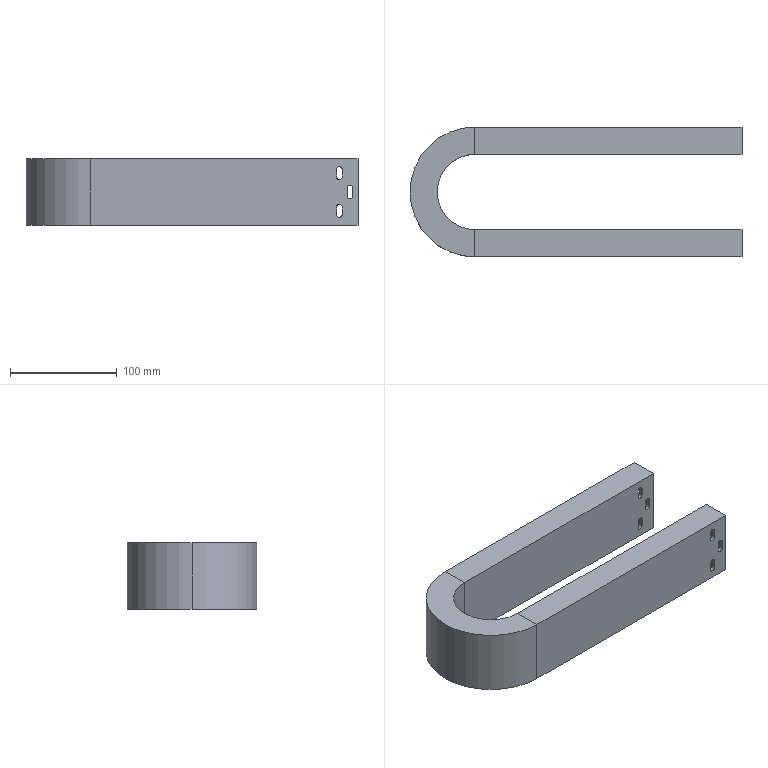Part | NX | features BREP 1 | 1 solid | 84 faces | box 310.75 x 121.5 x 62 mm | volume 440552 mm3 | plane 46 | cylinder 38 | commonest cylinder face diameters 5.2 x30 70.5 x2 78 x2 114 x2 121.5 x2